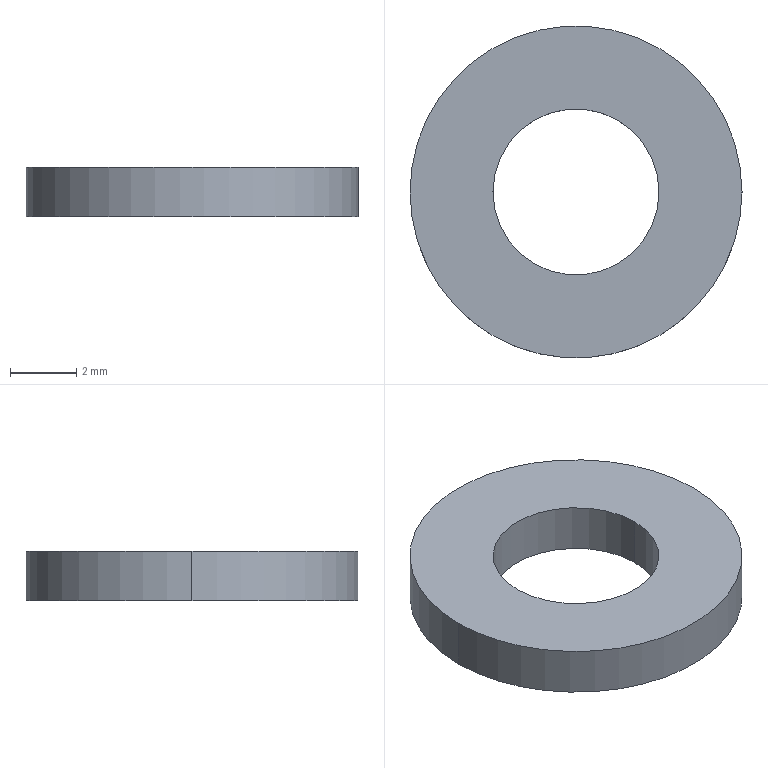Part | SolidWorks | features Extrusion 1 | 1 solid | 6 faces | box 10 x 10 x 1.5 mm | volume 88.357 mm3 | cylinder 4 | plane 2 | commonest cylinder face diameters 5 x2 10 x2
STEP:
#1=CARTESIAN_POINT('',(-2.5,0.,1.5));
#2=VERTEX_POINT('',#1);
#3=CARTESIAN_POINT('',(2.5,0.,1.5));
#4=VERTEX_POINT('',#3);
#5=CARTESIAN_POINT('',(0.,0.,1.5));
#6=DIRECTION('',(0.,0.,1.));
#7=DIRECTION('',(1.,0.,0.));
#8=AXIS2_PLACEMENT_3D('',#5,#6,#7);
#9=CIRCLE('',#8,2.5);
#10=EDGE_CURVE('',#2,#4,#9,.T.);
#11=ORIENTED_EDGE('',*,*,#10,.T.);
#12=CARTESIAN_POINT('',(2.5,0.,0.));
#13=VERTEX_POINT('',#12);
#14=CARTESIAN_POINT('',(2.5,0.,1.5));
#15=DIRECTION('',(0.,0.,-1.));
#16=VECTOR('',#15,1000.);
#17=LINE('',#14,#16);
#18=EDGE_CURVE('',#4,#13,#17,.T.);
#19=ORIENTED_EDGE('',*,*,#18,.T.);
#20=CARTESIAN_POINT('',(-2.5,0.,0.));
#21=VERTEX_POINT('',#20);
#22=CARTESIAN_POINT('',(0.,0.,0.));
#23=DIRECTION('',(0.,0.,1.));
#24=DIRECTION('',(1.,0.,0.));
#25=AXIS2_PLACEMENT_3D('',#22,#23,#24);
#26=CIRCLE('',#25,2.5);
#27=EDGE_CURVE('',#21,#13,#26,.T.);
#28=ORIENTED_EDGE('',*,*,#27,.F.);
#29=CARTESIAN_POINT('',(-2.5,0.,1.5));
#30=DIRECTION('',(0.,0.,-1.));
#31=VECTOR('',#30,1000.);
#32=LINE('',#29,#31);
#33=EDGE_CURVE('',#2,#21,#32,.T.);
#34=ORIENTED_EDGE('',*,*,#33,.F.);
#35=EDGE_LOOP('',(#11,#19,#28,#34));
#36=FACE_OUTER_BOUND('',#35,.T.);
#37=CARTESIAN_POINT('',(0.,0.,1.5));
#38=DIRECTION('',(0.,0.,-1.));
#39=DIRECTION('',(-1.,0.,0.));
#40=AXIS2_PLACEMENT_3D('',#37,#38,#39);
#41=CYLINDRICAL_SURFACE('',#40,2.5);
#42=ADVANCED_FACE('',(#36),#41,.F.);
#43=CARTESIAN_POINT('',(5.,0.,1.5));
#44=VERTEX_POINT('',#43);
#45=CARTESIAN_POINT('',(-5.,0.,1.5));
#46=VERTEX_POINT('',#45);
#47=CARTESIAN_POINT('',(0.,0.,1.5));
#48=DIRECTION('',(0.,0.,1.));
#49=DIRECTION('',(1.,0.,0.));
#50=AXIS2_PLACEMENT_3D('',#47,#48,#49);
#51=CIRCLE('',#50,5.);
#52=EDGE_CURVE('',#44,#46,#51,.T.);
#53=ORIENTED_EDGE('',*,*,#52,.F.);
#54=CARTESIAN_POINT('',(5.,0.,0.));
#55=VERTEX_POINT('',#54);
#56=CARTESIAN_POINT('',(5.,0.,1.5));
#57=DIRECTION('',(0.,0.,-1.));
#58=VECTOR('',#57,1000.);
#59=LINE('',#56,#58);
#60=EDGE_CURVE('',#44,#55,#59,.T.);
#61=ORIENTED_EDGE('',*,*,#60,.T.);
#62=CARTESIAN_POINT('',(-5.,0.,0.));
#63=VERTEX_POINT('',#62);
#64=CARTESIAN_POINT('',(0.,0.,0.));
#65=DIRECTION('',(0.,0.,1.));
#66=DIRECTION('',(1.,0.,0.));
#67=AXIS2_PLACEMENT_3D('',#64,#65,#66);
#68=CIRCLE('',#67,5.);
#69=EDGE_CURVE('',#55,#63,#68,.T.);
#70=ORIENTED_EDGE('',*,*,#69,.T.);
#71=CARTESIAN_POINT('',(-5.,0.,1.5));
#72=DIRECTION('',(0.,0.,-1.));
#73=VECTOR('',#72,1000.);
#74=LINE('',#71,#73);
#75=EDGE_CURVE('',#46,#63,#74,.T.);
#76=ORIENTED_EDGE('',*,*,#75,.F.);
#77=EDGE_LOOP('',(#53,#61,#70,#76));
#78=FACE_OUTER_BOUND('',#77,.T.);
#79=CARTESIAN_POINT('',(0.,0.,1.5));
#80=DIRECTION('',(0.,0.,-1.));
#81=DIRECTION('',(-1.,0.,0.));
#82=AXIS2_PLACEMENT_3D('',#79,#80,#81);
#83=CYLINDRICAL_SURFACE('',#82,5.);
#84=ADVANCED_FACE('',(#78),#83,.T.);
#85=CARTESIAN_POINT('',(0.,0.,1.5));
#86=DIRECTION('',(0.,0.,1.));
#87=DIRECTION('',(1.,0.,0.));
#88=AXIS2_PLACEMENT_3D('',#85,#86,#87);
#89=CIRCLE('',#88,5.);
#90=EDGE_CURVE('',#46,#44,#89,.T.);
#91=ORIENTED_EDGE('',*,*,#90,.T.);
#92=ORIENTED_EDGE('',*,*,#52,.T.);
#93=EDGE_LOOP('',(#91,#92));
#94=FACE_OUTER_BOUND('',#93,.T.);
#95=ORIENTED_EDGE('',*,*,#10,.F.);
#96=CARTESIAN_POINT('',(0.,0.,1.5));
#97=DIRECTION('',(0.,0.,1.));
#98=DIRECTION('',(1.,0.,0.));
#99=AXIS2_PLACEMENT_3D('',#96,#97,#98);
#100=CIRCLE('',#99,2.5);
#101=EDGE_CURVE('',#4,#2,#100,.T.);
#102=ORIENTED_EDGE('',*,*,#101,.F.);
#103=EDGE_LOOP('',(#95,#102));
#104=FACE_BOUND('',#103,.T.);
#105=CARTESIAN_POINT('',(0.,0.,1.5));
#106=DIRECTION('',(0.,0.,1.));
#107=DIRECTION('',(1.,0.,0.));
#108=AXIS2_PLACEMENT_3D('',#105,#106,#107);
#109=PLANE('',#108);
#110=ADVANCED_FACE('',(#94,#104),#109,.T.);
#111=CARTESIAN_POINT('',(0.,0.,0.));
#112=DIRECTION('',(0.,0.,1.));
#113=DIRECTION('',(1.,0.,0.));
#114=AXIS2_PLACEMENT_3D('',#111,#112,#113);
#115=CIRCLE('',#114,5.);
#116=EDGE_CURVE('',#63,#55,#115,.T.);
#117=ORIENTED_EDGE('',*,*,#116,.F.);
#118=ORIENTED_EDGE('',*,*,#69,.F.);
#119=EDGE_LOOP('',(#117,#118));
#120=FACE_OUTER_BOUND('',#119,.T.);
#121=ORIENTED_EDGE('',*,*,#27,.T.);
#122=CARTESIAN_POINT('',(0.,0.,0.));
#123=DIRECTION('',(0.,0.,1.));
#124=DIRECTION('',(1.,0.,0.));
#125=AXIS2_PLACEMENT_3D('',#122,#123,#124);
#126=CIRCLE('',#125,2.5);
#127=EDGE_CURVE('',#13,#21,#126,.T.);
#128=ORIENTED_EDGE('',*,*,#127,.T.);
#129=EDGE_LOOP('',(#121,#128));
#130=FACE_BOUND('',#129,.T.);
#131=CARTESIAN_POINT('',(0.,0.,0.));
#132=DIRECTION('',(0.,0.,1.));
#133=DIRECTION('',(1.,0.,0.));
#134=AXIS2_PLACEMENT_3D('',#131,#132,#133);
#135=PLANE('',#134);
#136=ADVANCED_FACE('',(#120,#130),#135,.F.);
#137=ORIENTED_EDGE('',*,*,#60,.F.);
#138=ORIENTED_EDGE('',*,*,#90,.F.);
#139=ORIENTED_EDGE('',*,*,#75,.T.);
#140=ORIENTED_EDGE('',*,*,#116,.T.);
#141=EDGE_LOOP('',(#137,#138,#139,#140));
#142=FACE_OUTER_BOUND('',#141,.T.);
#143=CARTESIAN_POINT('',(0.,0.,1.5));
#144=DIRECTION('',(0.,0.,-1.));
#145=DIRECTION('',(-1.,0.,0.));
#146=AXIS2_PLACEMENT_3D('',#143,#144,#145);
#147=CYLINDRICAL_SURFACE('',#146,5.);
#148=ADVANCED_FACE('',(#142),#147,.T.);
#149=ORIENTED_EDGE('',*,*,#18,.F.);
#150=ORIENTED_EDGE('',*,*,#101,.T.);
#151=ORIENTED_EDGE('',*,*,#33,.T.);
#152=ORIENTED_EDGE('',*,*,#127,.F.);
#153=EDGE_LOOP('',(#149,#150,#151,#152));
#154=FACE_OUTER_BOUND('',#153,.T.);
#155=CARTESIAN_POINT('',(0.,0.,1.5));
#156=DIRECTION('',(0.,0.,-1.));
#157=DIRECTION('',(-1.,0.,0.));
#158=AXIS2_PLACEMENT_3D('',#155,#156,#157);
#159=CYLINDRICAL_SURFACE('',#158,2.5);
#160=ADVANCED_FACE('',(#154),#159,.F.);
#161=CLOSED_SHELL('',(#42,#84,#110,#136,#148,#160));
#162=MANIFOLD_SOLID_BREP('',#161);
#163=CARTESIAN_POINT('',(0.,0.,0.));
#164=DIRECTION('',(0.,0.,1.));
#165=DIRECTION('',(1.,0.,0.));
#166=AXIS2_PLACEMENT_3D('',#163,#164,#165);
#167=(LENGTH_UNIT()NAMED_UNIT(*)SI_UNIT(.MILLI.,.METRE.));
#168=UNCERTAINTY_MEASURE_WITH_UNIT(LENGTH_MEASURE(0.00001),#167,'','');
#169=(NAMED_UNIT(*)PLANE_ANGLE_UNIT()SI_UNIT($,.RADIAN.));
#170=(NAMED_UNIT(*)SI_UNIT($,.STERADIAN.)SOLID_ANGLE_UNIT());
#171=(GEOMETRIC_REPRESENTATION_CONTEXT(3)GLOBAL_UNCERTAINTY_ASSIGNED_CONTEXT((#168))GLOBAL_UNIT_ASSIGNED_CONTEXT((#167,#169,#170))REPRESENTATION_CONTEXT('',''));
#172=ADVANCED_BREP_SHAPE_REPRESENTATION('',(#162,#166),#171);